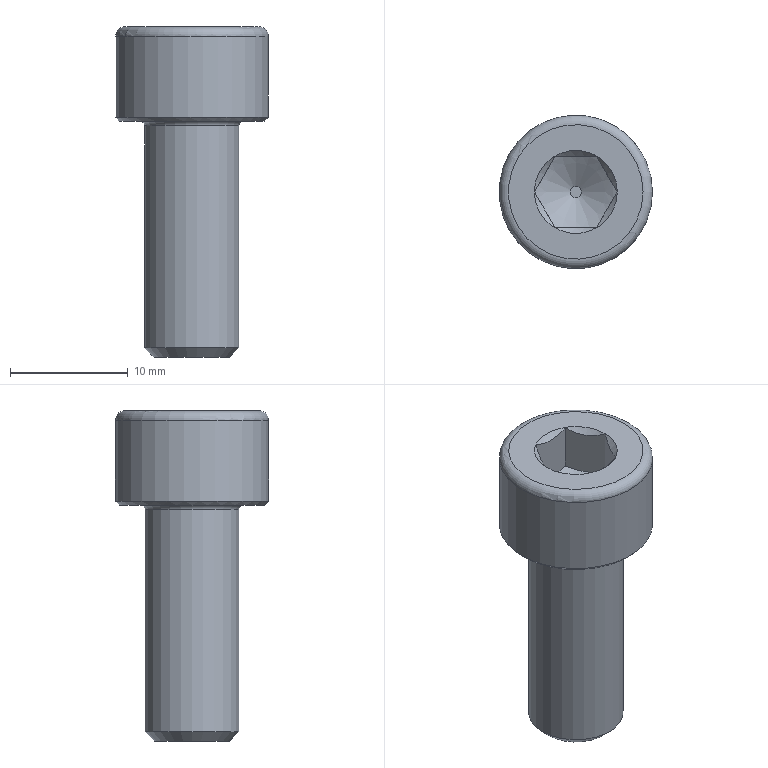Part | STEP file | Left | 1 solid | 18 faces | box 13 x 13 x 28 mm | volume 1899 mm3 | plane 10 | cone 4 | torus 2 | cylinder 2 | commonest cylinder face diameters 8 x1 13 x1
STEP:
#1=CARTESIAN_POINT('',(0.,0.,0.));
#2=DIRECTION('',(0.,0.,1.));
#3=DIRECTION('',(1.,0.,0.));
#4=AXIS2_PLACEMENT_3D('',#1,#2,#3);
#5=CARTESIAN_POINT('',(5.7,0.,8.));
#6=VERTEX_POINT('',#5);
#7=CARTESIAN_POINT('',(0.,0.,8.));
#8=DIRECTION('',(0.,0.,1.));
#9=DIRECTION('',(1.,0.,0.));
#10=AXIS2_PLACEMENT_3D('',#7,#8,#9);
#11=CIRCLE('',#10,5.7);
#12=CARTESIAN_POINT('',(0.,0.,8.));
#13=DIRECTION('',(0.,0.,1.));
#14=DIRECTION('',(1.,0.,0.));
#15=AXIS2_PLACEMENT_3D('',#12,#13,#14);
#16=PLANE('',#15);
#17=CARTESIAN_POINT('',(0.,0.));
#18=DIRECTION('',(1.,0.));
#19=AXIS2_PLACEMENT_2D('',#17,#18);
#20=CIRCLE('',#19,5.7);
#21=(GEOMETRIC_REPRESENTATION_CONTEXT(2)PARAMETRIC_REPRESENTATION_CONTEXT()REPRESENTATION_CONTEXT('',''));
#22=DEFINITIONAL_REPRESENTATION('',(#20),#21);
#23=PCURVE('',#16,#22);
#24=CARTESIAN_POINT('',(0.,0.,7.2));
#25=DIRECTION('',(0.,0.,-1.));
#26=DIRECTION('',(1.,0.,0.));
#27=AXIS2_PLACEMENT_3D('',#24,#25,#26);
#28=TOROIDAL_SURFACE('',#27,5.7,0.8);
#29=CARTESIAN_POINT('',(6.283,4.712));
#30=DIRECTION('',(-1.,0.));
#31=VECTOR('',#30,1.);
#32=LINE('',#29,#31);
#33=(GEOMETRIC_REPRESENTATION_CONTEXT(2)PARAMETRIC_REPRESENTATION_CONTEXT()REPRESENTATION_CONTEXT('',''));
#34=DEFINITIONAL_REPRESENTATION('',(#32),#33);
#35=PCURVE('',#28,#34);
#36=SURFACE_CURVE('',#11,(#23,#35),.PCURVE_S1.);
#37=EDGE_CURVE('',#6,#6,#36,.T.);
#38=ORIENTED_EDGE('',*,*,#37,.F.);
#39=EDGE_LOOP('',(#38));
#40=FACE_BOUND('',#39,.F.);
#41=CARTESIAN_POINT('',(-3.516,0.,8.));
#42=VERTEX_POINT('',#41);
#43=CARTESIAN_POINT('',(0.,0.,8.));
#44=DIRECTION('',(0.,0.,-1.));
#45=DIRECTION('',(-1.,0.,0.));
#46=AXIS2_PLACEMENT_3D('',#43,#44,#45);
#47=CIRCLE('',#46,3.516);
#48=CARTESIAN_POINT('',(-3.516,0.));
#49=CARTESIAN_POINT('',(-3.516,6.09));
#50=CARTESIAN_POINT('',(1.758,3.045));
#51=CARTESIAN_POINT('',(7.032,0.));
#52=CARTESIAN_POINT('',(1.758,-3.045));
#53=CARTESIAN_POINT('',(-3.516,-6.09));
#54=CARTESIAN_POINT('',(-3.516,0.));
#55=(BOUNDED_CURVE()B_SPLINE_CURVE(2,(#48,#49,#50,#51,#52,#53,#54),.UNSPECIFIED.,.T.,.F.)B_SPLINE_CURVE_WITH_KNOTS((1,2,2,2,2,1),(-2.094,0.,2.094,4.189,6.283,8.378),.UNSPECIFIED.)CURVE()GEOMETRIC_REPRESENTATION_ITEM()RATIONAL_B_SPLINE_CURVE((1.,0.5,1.,0.5,1.,0.5,1.))REPRESENTATION_ITEM(''));
#56=(GEOMETRIC_REPRESENTATION_CONTEXT(2)PARAMETRIC_REPRESENTATION_CONTEXT()REPRESENTATION_CONTEXT('',''));
#57=DEFINITIONAL_REPRESENTATION('',(#55),#56);
#58=PCURVE('',#16,#57);
#59=CARTESIAN_POINT('',(0.,0.,12.));
#60=DIRECTION('',(0.,0.,1.));
#61=DIRECTION('',(-1.,0.,0.));
#62=AXIS2_PLACEMENT_3D('',#59,#60,#61);
#63=CONICAL_SURFACE('',#62,7.516,0.7854);
#64=CARTESIAN_POINT('',(6.283,-4.));
#65=DIRECTION('',(-1.,0.));
#66=VECTOR('',#65,1.);
#67=LINE('',#64,#66);
#68=(GEOMETRIC_REPRESENTATION_CONTEXT(2)PARAMETRIC_REPRESENTATION_CONTEXT()REPRESENTATION_CONTEXT('',''));
#69=DEFINITIONAL_REPRESENTATION('',(#67),#68);
#70=PCURVE('',#63,#69);
#71=SURFACE_CURVE('',#47,(#58,#70),.PCURVE_S1.);
#72=EDGE_CURVE('',#42,#42,#71,.T.);
#73=ORIENTED_EDGE('',*,*,#72,.F.);
#74=EDGE_LOOP('',(#73));
#75=FACE_BOUND('',#74,.F.);
#76=ADVANCED_FACE('',(#40,#75),#16,.T.);
#77=CARTESIAN_POINT('',(6.5,0.,7.2));
#78=VERTEX_POINT('',#77);
#79=CARTESIAN_POINT('',(5.7,0.,7.2));
#80=DIRECTION('',(0.,1.,0.));
#81=DIRECTION('',(0.,0.,1.));
#82=AXIS2_PLACEMENT_3D('',#79,#80,#81);
#83=CIRCLE('',#82,0.8);
#84=CARTESIAN_POINT('',(6.283,4.712));
#85=DIRECTION('',(0.,1.));
#86=VECTOR('',#85,1.);
#87=LINE('',#84,#86);
#88=(GEOMETRIC_REPRESENTATION_CONTEXT(2)PARAMETRIC_REPRESENTATION_CONTEXT()REPRESENTATION_CONTEXT('',''));
#89=DEFINITIONAL_REPRESENTATION('',(#87),#88);
#90=PCURVE('',#28,#89);
#91=CARTESIAN_POINT('',(0.,4.712));
#92=DIRECTION('',(0.,1.));
#93=VECTOR('',#92,1.);
#94=LINE('',#91,#93);
#95=(GEOMETRIC_REPRESENTATION_CONTEXT(2)PARAMETRIC_REPRESENTATION_CONTEXT()REPRESENTATION_CONTEXT('',''));
#96=DEFINITIONAL_REPRESENTATION('',(#94),#95);
#97=PCURVE('',#28,#96);
#98=SEAM_CURVE('',#83,(#90,#97),.PCURVE_S1.);
#99=EDGE_CURVE('',#6,#78,#98,.T.);
#100=ORIENTED_EDGE('',*,*,#99,.T.);
#101=CARTESIAN_POINT('',(0.,0.,7.2));
#102=DIRECTION('',(0.,0.,1.));
#103=DIRECTION('',(1.,0.,0.));
#104=AXIS2_PLACEMENT_3D('',#101,#102,#103);
#105=CIRCLE('',#104,6.5);
#106=CARTESIAN_POINT('',(6.283,6.283));
#107=DIRECTION('',(-1.,0.));
#108=VECTOR('',#107,1.);
#109=LINE('',#106,#108);
#110=(GEOMETRIC_REPRESENTATION_CONTEXT(2)PARAMETRIC_REPRESENTATION_CONTEXT()REPRESENTATION_CONTEXT('',''));
#111=DEFINITIONAL_REPRESENTATION('',(#109),#110);
#112=PCURVE('',#28,#111);
#113=CARTESIAN_POINT('',(0.,0.,7.2));
#114=DIRECTION('',(0.,0.,-1.));
#115=DIRECTION('',(1.,0.,0.));
#116=AXIS2_PLACEMENT_3D('',#113,#114,#115);
#117=CYLINDRICAL_SURFACE('',#116,6.5);
#118=CARTESIAN_POINT('',(6.283,0.));
#119=DIRECTION('',(-1.,0.));
#120=VECTOR('',#119,1.);
#121=LINE('',#118,#120);
#122=(GEOMETRIC_REPRESENTATION_CONTEXT(2)PARAMETRIC_REPRESENTATION_CONTEXT()REPRESENTATION_CONTEXT('',''));
#123=DEFINITIONAL_REPRESENTATION('',(#121),#122);
#124=PCURVE('',#117,#123);
#125=SURFACE_CURVE('',#105,(#112,#124),.PCURVE_S1.);
#126=EDGE_CURVE('',#78,#78,#125,.T.);
#127=ORIENTED_EDGE('',*,*,#126,.T.);
#128=ORIENTED_EDGE('',*,*,#99,.F.);
#129=ORIENTED_EDGE('',*,*,#37,.F.);
#130=EDGE_LOOP('',(#100,#127,#128,#129));
#131=FACE_BOUND('',#130,.T.);
#132=ADVANCED_FACE('',(#131),#28,.T.);
#133=CARTESIAN_POINT('',(1.749,3.03,7.983));
#134=VERTEX_POINT('',#133);
#135=CARTESIAN_POINT('',(-1.749,3.03,7.983));
#136=VERTEX_POINT('',#135);
#137=CARTESIAN_POINT('',(0.,3.03,4.484));
#138=DIRECTION('',(0.,-1.,0.));
#139=DIRECTION('',(0.,0.,1.));
#140=AXIS2_PLACEMENT_3D('',#137,#138,#139);
#141=HYPERBOLA('',#140,3.03,3.03);
#142=CARTESIAN_POINT('',(4.189,-4.017));
#143=CARTESIAN_POINT('',(4.203,-4.047));
#144=CARTESIAN_POINT('',(4.232,-4.102));
#145=CARTESIAN_POINT('',(4.277,-4.176));
#146=CARTESIAN_POINT('',(4.323,-4.243));
#147=CARTESIAN_POINT('',(4.37,-4.301));
#148=CARTESIAN_POINT('',(4.417,-4.351));
#149=CARTESIAN_POINT('',(4.465,-4.393));
#150=CARTESIAN_POINT('',(4.514,-4.427));
#151=CARTESIAN_POINT('',(4.563,-4.453));
#152=CARTESIAN_POINT('',(4.613,-4.472));
#153=CARTESIAN_POINT('',(4.662,-4.484));
#154=CARTESIAN_POINT('',(4.712,-4.487));
#155=CARTESIAN_POINT('',(4.762,-4.484));
#156=CARTESIAN_POINT('',(4.812,-4.472));
#157=CARTESIAN_POINT('',(4.862,-4.453));
#158=CARTESIAN_POINT('',(4.911,-4.427));
#159=CARTESIAN_POINT('',(4.96,-4.393));
#160=CARTESIAN_POINT('',(5.008,-4.351));
#161=CARTESIAN_POINT('',(5.055,-4.301));
#162=CARTESIAN_POINT('',(5.102,-4.243));
#163=CARTESIAN_POINT('',(5.148,-4.176));
#164=CARTESIAN_POINT('',(5.192,-4.102));
#165=CARTESIAN_POINT('',(5.222,-4.047));
#166=CARTESIAN_POINT('',(5.236,-4.017));
#167=B_SPLINE_CURVE_WITH_KNOTS('',3,(#142,#143,#144,#145,#146,#147,#148,#149,#150,#151,#152,#153,#154,#155,#156,#157,#158,#159,#160,#161,#162,#163,#164,#165,#166),.UNSPECIFIED.,.F.,.F.,(4,1,1,1,1,1,1,1,1,1,1,1,1,1,1,1,1,1,1,1,1,1,4),(-0.5493,-0.4994,-0.4494,-0.3995,-0.3496,-0.2996,-0.2497,-0.1997,-0.1498,-0.09987,-0.04994,0.,0.04994,0.09987,0.1498,0.1997,0.2497,0.2996,0.3496,0.3995,0.4494,0.4994,0.5493),.UNSPECIFIED.);
#168=(GEOMETRIC_REPRESENTATION_CONTEXT(2)PARAMETRIC_REPRESENTATION_CONTEXT()REPRESENTATION_CONTEXT('',''));
#169=DEFINITIONAL_REPRESENTATION('',(#167),#168);
#170=PCURVE('',#63,#169);
#171=CARTESIAN_POINT('',(-1.749,3.03,12.));
#172=DIRECTION('',(0.,-1.,0.));
#173=DIRECTION('',(1.,0.,0.));
#174=AXIS2_PLACEMENT_3D('',#171,#172,#173);
#175=PLANE('',#174);
#176=CARTESIAN_POINT('',(1.749,-7.516));
#177=DIRECTION('',(0.,1.));
#178=AXIS2_PLACEMENT_2D('',#176,#177);
#179=HYPERBOLA('',#178,3.03,3.03);
#180=(GEOMETRIC_REPRESENTATION_CONTEXT(2)PARAMETRIC_REPRESENTATION_CONTEXT()REPRESENTATION_CONTEXT('',''));
#181=DEFINITIONAL_REPRESENTATION('',(#179),#180);
#182=PCURVE('',#175,#181);
#183=SURFACE_CURVE('',#141,(#170,#182),.PCURVE_S1.);
#184=EDGE_CURVE('',#134,#136,#183,.T.);
#185=ORIENTED_EDGE('',*,*,#184,.T.);
#186=CARTESIAN_POINT('',(-3.499,0.,7.983));
#187=VERTEX_POINT('',#186);
#188=CARTESIAN_POINT('',(-2.624,1.515,4.484));
#189=DIRECTION('',(0.866,-0.5,0.));
#190=DIRECTION('',(0.,0.,1.));
#191=AXIS2_PLACEMENT_3D('',#188,#189,#190);
#192=HYPERBOLA('',#191,3.03,3.03);
#193=CARTESIAN_POINT('',(5.236,-4.017));
#194=CARTESIAN_POINT('',(5.25,-4.047));
#195=CARTESIAN_POINT('',(5.28,-4.102));
#196=CARTESIAN_POINT('',(5.324,-4.176));
#197=CARTESIAN_POINT('',(5.37,-4.243));
#198=CARTESIAN_POINT('',(5.417,-4.301));
#199=CARTESIAN_POINT('',(5.464,-4.351));
#200=CARTESIAN_POINT('',(5.512,-4.393));
#201=CARTESIAN_POINT('',(5.561,-4.427));
#202=CARTESIAN_POINT('',(5.61,-4.453));
#203=CARTESIAN_POINT('',(5.66,-4.472));
#204=CARTESIAN_POINT('',(5.71,-4.484));
#205=CARTESIAN_POINT('',(5.76,-4.487));
#206=CARTESIAN_POINT('',(5.81,-4.484));
#207=CARTESIAN_POINT('',(5.859,-4.472));
#208=CARTESIAN_POINT('',(5.909,-4.453));
#209=CARTESIAN_POINT('',(5.958,-4.427));
#210=CARTESIAN_POINT('',(6.007,-4.393));
#211=CARTESIAN_POINT('',(6.055,-4.351));
#212=CARTESIAN_POINT('',(6.102,-4.301));
#213=CARTESIAN_POINT('',(6.149,-4.243));
#214=CARTESIAN_POINT('',(6.195,-4.176));
#215=CARTESIAN_POINT('',(6.24,-4.102));
#216=CARTESIAN_POINT('',(6.269,-4.047));
#217=CARTESIAN_POINT('',(6.283,-4.017));
#218=B_SPLINE_CURVE_WITH_KNOTS('',3,(#193,#194,#195,#196,#197,#198,#199,#200,#201,#202,#203,#204,#205,#206,#207,#208,#209,#210,#211,#212,#213,#214,#215,#216,#217),.UNSPECIFIED.,.F.,.F.,(4,1,1,1,1,1,1,1,1,1,1,1,1,1,1,1,1,1,1,1,1,1,4),(-0.5493,-0.4994,-0.4494,-0.3995,-0.3496,-0.2996,-0.2497,-0.1997,-0.1498,-0.09987,-0.04994,0.,0.04994,0.09987,0.1498,0.1997,0.2497,0.2996,0.3496,0.3995,0.4494,0.4994,0.5493),.UNSPECIFIED.);
#219=(GEOMETRIC_REPRESENTATION_CONTEXT(2)PARAMETRIC_REPRESENTATION_CONTEXT()REPRESENTATION_CONTEXT('',''));
#220=DEFINITIONAL_REPRESENTATION('',(#218),#219);
#221=PCURVE('',#63,#220);
#222=CARTESIAN_POINT('',(-3.499,0.,12.));
#223=DIRECTION('',(0.866,-0.5,0.));
#224=DIRECTION('',(0.5,0.866,0.));
#225=AXIS2_PLACEMENT_3D('',#222,#223,#224);
#226=PLANE('',#225);
#227=CARTESIAN_POINT('',(1.749,-7.516));
#228=DIRECTION('',(0.,1.));
#229=AXIS2_PLACEMENT_2D('',#227,#228);
#230=HYPERBOLA('',#229,3.03,3.03);
#231=(GEOMETRIC_REPRESENTATION_CONTEXT(2)PARAMETRIC_REPRESENTATION_CONTEXT()REPRESENTATION_CONTEXT('',''));
#232=DEFINITIONAL_REPRESENTATION('',(#230),#231);
#233=PCURVE('',#226,#232);
#234=SURFACE_CURVE('',#192,(#221,#233),.PCURVE_S1.);
#235=EDGE_CURVE('',#136,#187,#234,.T.);
#236=ORIENTED_EDGE('',*,*,#235,.T.);
#237=CARTESIAN_POINT('',(-7.516,0.,12.));
#238=DIRECTION('',(0.7071,0.,-0.7071));
#239=VECTOR('',#238,1.);
#240=LINE('',#237,#239);
#241=CARTESIAN_POINT('',(6.283,0.));
#242=DIRECTION('',(0.,-1.));
#243=VECTOR('',#242,1.);
#244=LINE('',#241,#243);
#245=(GEOMETRIC_REPRESENTATION_CONTEXT(2)PARAMETRIC_REPRESENTATION_CONTEXT()REPRESENTATION_CONTEXT('',''));
#246=DEFINITIONAL_REPRESENTATION('',(#244),#245);
#247=PCURVE('',#63,#246);
#248=CARTESIAN_POINT('',(0.,0.));
#249=DIRECTION('',(0.,-1.));
#250=VECTOR('',#249,1.);
#251=LINE('',#248,#250);
#252=(GEOMETRIC_REPRESENTATION_CONTEXT(2)PARAMETRIC_REPRESENTATION_CONTEXT()REPRESENTATION_CONTEXT('',''));
#253=DEFINITIONAL_REPRESENTATION('',(#251),#252);
#254=PCURVE('',#63,#253);
#255=SEAM_CURVE('',#240,(#247,#254),.PCURVE_S1.);
#256=EDGE_CURVE('',#42,#187,#255,.T.);
#257=ORIENTED_EDGE('',*,*,#256,.F.);
#258=ORIENTED_EDGE('',*,*,#72,.T.);
#259=ORIENTED_EDGE('',*,*,#256,.T.);
#260=CARTESIAN_POINT('',(-1.749,-3.03,7.983));
#261=VERTEX_POINT('',#260);
#262=CARTESIAN_POINT('',(-2.624,-1.515,4.484));
#263=DIRECTION('',(0.866,0.5,0.));
#264=DIRECTION('',(0.,0.,1.));
#265=AXIS2_PLACEMENT_3D('',#262,#263,#264);
#266=HYPERBOLA('',#265,3.03,3.03);
#267=CARTESIAN_POINT('',(0.,-4.017));
#268=CARTESIAN_POINT('',(0.01441,-4.047));
#269=CARTESIAN_POINT('',(0.04361,-4.102));
#270=CARTESIAN_POINT('',(0.08842,-4.176));
#271=CARTESIAN_POINT('',(0.1342,-4.243));
#272=CARTESIAN_POINT('',(0.1808,-4.301));
#273=CARTESIAN_POINT('',(0.2282,-4.351));
#274=CARTESIAN_POINT('',(0.2764,-4.393));
#275=CARTESIAN_POINT('',(0.3251,-4.427));
#276=CARTESIAN_POINT('',(0.3743,-4.453));
#277=CARTESIAN_POINT('',(0.4238,-4.472));
#278=CARTESIAN_POINT('',(0.4737,-4.484));
#279=CARTESIAN_POINT('',(0.5236,-4.487));
#280=CARTESIAN_POINT('',(0.5735,-4.484));
#281=CARTESIAN_POINT('',(0.6233,-4.472));
#282=CARTESIAN_POINT('',(0.6729,-4.453));
#283=CARTESIAN_POINT('',(0.7221,-4.427));
#284=CARTESIAN_POINT('',(0.7708,-4.393));
#285=CARTESIAN_POINT('',(0.819,-4.351));
#286=CARTESIAN_POINT('',(0.8664,-4.301));
#287=CARTESIAN_POINT('',(0.913,-4.243));
#288=CARTESIAN_POINT('',(0.9588,-4.176));
#289=CARTESIAN_POINT('',(1.004,-4.102));
#290=CARTESIAN_POINT('',(1.033,-4.047));
#291=CARTESIAN_POINT('',(1.047,-4.017));
#292=B_SPLINE_CURVE_WITH_KNOTS('',3,(#267,#268,#269,#270,#271,#272,#273,#274,#275,#276,#277,#278,#279,#280,#281,#282,#283,#284,#285,#286,#287,#288,#289,#290,#291),.UNSPECIFIED.,.F.,.F.,(4,1,1,1,1,1,1,1,1,1,1,1,1,1,1,1,1,1,1,1,1,1,4),(-0.5493,-0.4994,-0.4494,-0.3995,-0.3496,-0.2996,-0.2497,-0.1997,-0.1498,-0.09987,-0.04994,0.,0.04994,0.09987,0.1498,0.1997,0.2497,0.2996,0.3496,0.3995,0.4494,0.4994,0.5493),.UNSPECIFIED.);
#293=(GEOMETRIC_REPRESENTATION_CONTEXT(2)PARAMETRIC_REPRESENTATION_CONTEXT()REPRESENTATION_CONTEXT('',''));
#294=DEFINITIONAL_REPRESENTATION('',(#292),#293);
#295=PCURVE('',#63,#294);
#296=CARTESIAN_POINT('',(-1.749,-3.03,12.));
#297=DIRECTION('',(0.866,0.5,0.));
#298=DIRECTION('',(-0.5,0.866,0.));
#299=AXIS2_PLACEMENT_3D('',#296,#297,#298);
#300=PLANE('',#299);
#301=CARTESIAN_POINT('',(1.749,-7.516));
#302=DIRECTION('',(0.,1.));
#303=AXIS2_PLACEMENT_2D('',#301,#302);
#304=HYPERBOLA('',#303,3.03,3.03);
#305=(GEOMETRIC_REPRESENTATION_CONTEXT(2)PARAMETRIC_REPRESENTATION_CONTEXT()REPRESENTATION_CONTEXT('',''));
#306=DEFINITIONAL_REPRESENTATION('',(#304),#305);
#307=PCURVE('',#300,#306);
#308=SURFACE_CURVE('',#266,(#295,#307),.PCURVE_S1.);
#309=EDGE_CURVE('',#187,#261,#308,.T.);
#310=ORIENTED_EDGE('',*,*,#309,.T.);
#311=CARTESIAN_POINT('',(1.749,-3.03,7.983));
#312=VERTEX_POINT('',#311);
#313=CARTESIAN_POINT('',(0.,-3.03,4.484));
#314=DIRECTION('',(0.,1.,0.));
#315=DIRECTION('',(0.,0.,1.));
#316=AXIS2_PLACEMENT_3D('',#313,#314,#315);
#317=HYPERBOLA('',#316,3.03,3.03);
#318=CARTESIAN_POINT('',(1.047,-4.017));
#319=CARTESIAN_POINT('',(1.062,-4.047));
#320=CARTESIAN_POINT('',(1.091,-4.102));
#321=CARTESIAN_POINT('',(1.136,-4.176));
#322=CARTESIAN_POINT('',(1.181,-4.243));
#323=CARTESIAN_POINT('',(1.228,-4.301));
#324=CARTESIAN_POINT('',(1.275,-4.351));
#325=CARTESIAN_POINT('',(1.324,-4.393));
#326=CARTESIAN_POINT('',(1.372,-4.427));
#327=CARTESIAN_POINT('',(1.421,-4.453));
#328=CARTESIAN_POINT('',(1.471,-4.472));
#329=CARTESIAN_POINT('',(1.521,-4.484));
#330=CARTESIAN_POINT('',(1.571,-4.487));
#331=CARTESIAN_POINT('',(1.621,-4.484));
#332=CARTESIAN_POINT('',(1.671,-4.472));
#333=CARTESIAN_POINT('',(1.72,-4.453));
#334=CARTESIAN_POINT('',(1.769,-4.427));
#335=CARTESIAN_POINT('',(1.818,-4.393));
#336=CARTESIAN_POINT('',(1.866,-4.351));
#337=CARTESIAN_POINT('',(1.914,-4.301));
#338=CARTESIAN_POINT('',(1.96,-4.243));
#339=CARTESIAN_POINT('',(2.006,-4.176));
#340=CARTESIAN_POINT('',(2.051,-4.102));
#341=CARTESIAN_POINT('',(2.08,-4.047));
#342=CARTESIAN_POINT('',(2.094,-4.017));
#343=B_SPLINE_CURVE_WITH_KNOTS('',3,(#318,#319,#320,#321,#322,#323,#324,#325,#326,#327,#328,#329,#330,#331,#332,#333,#334,#335,#336,#337,#338,#339,#340,#341,#342),.UNSPECIFIED.,.F.,.F.,(4,1,1,1,1,1,1,1,1,1,1,1,1,1,1,1,1,1,1,1,1,1,4),(-0.5493,-0.4994,-0.4494,-0.3995,-0.3496,-0.2996,-0.2497,-0.1997,-0.1498,-0.09987,-0.04994,0.,0.04994,0.09987,0.1498,0.1997,0.2497,0.2996,0.3496,0.3995,0.4494,0.4994,0.5493),.UNSPECIFIED.);
#344=(GEOMETRIC_REPRESENTATION_CONTEXT(2)PARAMETRIC_REPRESENTATION_CONTEXT()REPRESENTATION_CONTEXT('',''));
#345=DEFINITIONAL_REPRESENTATION('',(#343),#344);
#346=PCURVE('',#63,#345);
#347=CARTESIAN_POINT('',(1.749,-3.03,12.));
#348=DIRECTION('',(0.,1.,0.));
#349=DIRECTION('',(-1.,0.,0.));
#350=AXIS2_PLACEMENT_3D('',#347,#348,#349);
#351=PLANE('',#350);
#352=CARTESIAN_POINT('',(1.749,-7.516));
#353=DIRECTION('',(0.,1.));
#354=AXIS2_PLACEMENT_2D('',#352,#353);
#355=HYPERBOLA('',#354,3.03,3.03);
#356=(GEOMETRIC_REPRESENTATION_CONTEXT(2)PARAMETRIC_REPRESENTATION_CONTEXT()REPRESENTATION_CONTEXT('',''));
#357=DEFINITIONAL_REPRESENTATION('',(#355),#356);
#358=PCURVE('',#351,#357);
#359=SURFACE_CURVE('',#317,(#346,#358),.PCURVE_S1.);
#360=EDGE_CURVE('',#261,#312,#359,.T.);
#361=ORIENTED_EDGE('',*,*,#360,.T.);
#362=CARTESIAN_POINT('',(3.499,0.,7.983));
#363=VERTEX_POINT('',#362);
#364=CARTESIAN_POINT('',(2.624,-1.515,4.484));
#365=DIRECTION('',(-0.866,0.5,0.));
#366=DIRECTION('',(0.,0.,1.));
#367=AXIS2_PLACEMENT_3D('',#364,#365,#366);
#368=HYPERBOLA('',#367,3.03,3.03);
#369=CARTESIAN_POINT('',(2.094,-4.017));
#370=CARTESIAN_POINT('',(2.109,-4.047));
#371=CARTESIAN_POINT('',(2.138,-4.102));
#372=CARTESIAN_POINT('',(2.183,-4.176));
#373=CARTESIAN_POINT('',(2.229,-4.243));
#374=CARTESIAN_POINT('',(2.275,-4.301));
#375=CARTESIAN_POINT('',(2.323,-4.351));
#376=CARTESIAN_POINT('',(2.371,-4.393));
#377=CARTESIAN_POINT('',(2.419,-4.427));
#378=CARTESIAN_POINT('',(2.469,-4.453));
#379=CARTESIAN_POINT('',(2.518,-4.472));
#380=CARTESIAN_POINT('',(2.568,-4.484));
#381=CARTESIAN_POINT('',(2.618,-4.487));
#382=CARTESIAN_POINT('',(2.668,-4.484));
#383=CARTESIAN_POINT('',(2.718,-4.472));
#384=CARTESIAN_POINT('',(2.767,-4.453));
#385=CARTESIAN_POINT('',(2.817,-4.427));
#386=CARTESIAN_POINT('',(2.865,-4.393));
#387=CARTESIAN_POINT('',(2.913,-4.351));
#388=CARTESIAN_POINT('',(2.961,-4.301));
#389=CARTESIAN_POINT('',(3.007,-4.243));
#390=CARTESIAN_POINT('',(3.053,-4.176));
#391=CARTESIAN_POINT('',(3.098,-4.102));
#392=CARTESIAN_POINT('',(3.127,-4.047));
#393=CARTESIAN_POINT('',(3.142,-4.017));
#394=B_SPLINE_CURVE_WITH_KNOTS('',3,(#369,#370,#371,#372,#373,#374,#375,#376,#377,#378,#379,#380,#381,#382,#383,#384,#385,#386,#387,#388,#389,#390,#391,#392,#393),.UNSPECIFIED.,.F.,.F.,(4,1,1,1,1,1,1,1,1,1,1,1,1,1,1,1,1,1,1,1,1,1,4),(-0.5493,-0.4994,-0.4494,-0.3995,-0.3496,-0.2996,-0.2497,-0.1997,-0.1498,-0.09987,-0.04994,0.,0.04994,0.09987,0.1498,0.1997,0.2497,0.2996,0.3496,0.3995,0.4494,0.4994,0.5493),.UNSPECIFIED.);
#395=(GEOMETRIC_REPRESENTATION_CONTEXT(2)PARAMETRIC_REPRESENTATION_CONTEXT()REPRESENTATION_CONTEXT('',''));
#396=DEFINITIONAL_REPRESENTATION('',(#394),#395);
#397=PCURVE('',#63,#396);
#398=CARTESIAN_POINT('',(3.499,0.,12.));
#399=DIRECTION('',(-0.866,0.5,0.));
#400=DIRECTION('',(-0.5,-0.866,0.));
#401=AXIS2_PLACEMENT_3D('',#398,#399,#400);
#402=PLANE('',#401);
#403=CARTESIAN_POINT('',(1.749,-7.516));
#404=DIRECTION('',(0.,1.));
#405=AXIS2_PLACEMENT_2D('',#403,#404);
#406=HYPERBOLA('',#405,3.03,3.03);
#407=(GEOMETRIC_REPRESENTATION_CONTEXT(2)PARAMETRIC_REPRESENTATION_CONTEXT()REPRESENTATION_CONTEXT('',''));
#408=DEFINITIONAL_REPRESENTATION('',(#406),#407);
#409=PCURVE('',#402,#408);
#410=SURFACE_CURVE('',#368,(#397,#409),.PCURVE_S1.);
#411=EDGE_CURVE('',#312,#363,#410,.T.);
#412=ORIENTED_EDGE('',*,*,#411,.T.);
#413=CARTESIAN_POINT('',(2.624,1.515,4.484));
#414=DIRECTION('',(-0.866,-0.5,0.));
#415=DIRECTION('',(0.,0.,1.));
#416=AXIS2_PLACEMENT_3D('',#413,#414,#415);
#417=HYPERBOLA('',#416,3.03,3.03);
#418=CARTESIAN_POINT('',(3.142,-4.017));
#419=CARTESIAN_POINT('',(3.156,-4.047));
#420=CARTESIAN_POINT('',(3.185,-4.102));
#421=CARTESIAN_POINT('',(3.23,-4.176));
#422=CARTESIAN_POINT('',(3.276,-4.243));
#423=CARTESIAN_POINT('',(3.322,-4.301));
#424=CARTESIAN_POINT('',(3.37,-4.351));
#425=CARTESIAN_POINT('',(3.418,-4.393));
#426=CARTESIAN_POINT('',(3.467,-4.427));
#427=CARTESIAN_POINT('',(3.516,-4.453));
#428=CARTESIAN_POINT('',(3.565,-4.472));
#429=CARTESIAN_POINT('',(3.615,-4.484));
#430=CARTESIAN_POINT('',(3.665,-4.487));
#431=CARTESIAN_POINT('',(3.715,-4.484));
#432=CARTESIAN_POINT('',(3.765,-4.472));
#433=CARTESIAN_POINT('',(3.815,-4.453));
#434=CARTESIAN_POINT('',(3.864,-4.427));
#435=CARTESIAN_POINT('',(3.912,-4.393));
#436=CARTESIAN_POINT('',(3.961,-4.351));
#437=CARTESIAN_POINT('',(4.008,-4.301));
#438=CARTESIAN_POINT('',(4.055,-4.243));
#439=CARTESIAN_POINT('',(4.1,-4.176));
#440=CARTESIAN_POINT('',(4.145,-4.102));
#441=CARTESIAN_POINT('',(4.174,-4.047));
#442=CARTESIAN_POINT('',(4.189,-4.017));
#443=B_SPLINE_CURVE_WITH_KNOTS('',3,(#418,#419,#420,#421,#422,#423,#424,#425,#426,#427,#428,#429,#430,#431,#432,#433,#434,#435,#436,#437,#438,#439,#440,#441,#442),.UNSPECIFIED.,.F.,.F.,(4,1,1,1,1,1,1,1,1,1,1,1,1,1,1,1,1,1,1,1,1,1,4),(-0.5493,-0.4994,-0.4494,-0.3995,-0.3496,-0.2996,-0.2497,-0.1997,-0.1498,-0.09987,-0.04994,0.,0.04994,0.09987,0.1498,0.1997,0.2497,0.2996,0.3496,0.3995,0.4494,0.4994,0.5493),.UNSPECIFIED.);
#444=(GEOMETRIC_REPRESENTATION_CONTEXT(2)PARAMETRIC_REPRESENTATION_CONTEXT()REPRESENTATION_CONTEXT('',''));
#445=DEFINITIONAL_REPRESENTATION('',(#443),#444);
#446=PCURVE('',#63,#445);
#447=CARTESIAN_POINT('',(1.749,3.03,12.));
#448=DIRECTION('',(-0.866,-0.5,0.));
#449=DIRECTION('',(0.5,-0.866,0.));
#450=AXIS2_PLACEMENT_3D('',#447,#448,#449);
#451=PLANE('',#450);
#452=CARTESIAN_POINT('',(1.749,-7.516));
#453=DIRECTION('',(0.,1.));
#454=AXIS2_PLACEMENT_2D('',#452,#453);
#455=HYPERBOLA('',#454,3.03,3.03);
#456=(GEOMETRIC_REPRESENTATION_CONTEXT(2)PARAMETRIC_REPRESENTATION_CONTEXT()REPRESENTATION_CONTEXT('',''));
#457=DEFINITIONAL_REPRESENTATION('',(#455),#456);
#458=PCURVE('',#451,#457);
#459=SURFACE_CURVE('',#417,(#446,#458),.PCURVE_S1.);
#460=EDGE_CURVE('',#363,#134,#459,.T.);
#461=ORIENTED_EDGE('',*,*,#460,.T.);
#462=EDGE_LOOP('',(#185,#236,#257,#258,#259,#310,#361,#412,#461));
#463=FACE_BOUND('',#462,.F.);
#464=ADVANCED_FACE('',(#463),#63,.F.);
#465=CARTESIAN_POINT('',(6.5,0.,0.335));
#466=VERTEX_POINT('',#465);
#467=CARTESIAN_POINT('',(6.5,0.,7.2));
#468=DIRECTION('',(0.,0.,-1.));
#469=VECTOR('',#468,1.);
#470=LINE('',#467,#469);
#471=CARTESIAN_POINT('',(6.283,0.));
#472=DIRECTION('',(0.,1.));
#473=VECTOR('',#472,1.);
#474=LINE('',#471,#473);
#475=(GEOMETRIC_REPRESENTATION_CONTEXT(2)PARAMETRIC_REPRESENTATION_CONTEXT()REPRESENTATION_CONTEXT('',''));
#476=DEFINITIONAL_REPRESENTATION('',(#474),#475);
#477=PCURVE('',#117,#476);
#478=CARTESIAN_POINT('',(0.,0.));
#479=DIRECTION('',(0.,1.));
#480=VECTOR('',#479,1.);
#481=LINE('',#478,#480);
#482=(GEOMETRIC_REPRESENTATION_CONTEXT(2)PARAMETRIC_REPRESENTATION_CONTEXT()REPRESENTATION_CONTEXT('',''));
#483=DEFINITIONAL_REPRESENTATION('',(#481),#482);
#484=PCURVE('',#117,#483);
#485=SEAM_CURVE('',#470,(#477,#484),.PCURVE_S1.);
#486=EDGE_CURVE('',#78,#466,#485,.T.);
#487=ORIENTED_EDGE('',*,*,#486,.T.);
#488=CARTESIAN_POINT('',(0.,0.,0.335));
#489=DIRECTION('',(0.,0.,1.));
#490=DIRECTION('',(1.,0.,0.));
#491=AXIS2_PLACEMENT_3D('',#488,#489,#490);
#492=CIRCLE('',#491,6.5);
#493=CARTESIAN_POINT('',(6.283,6.865));
#494=DIRECTION('',(-1.,0.));
#495=VECTOR('',#494,1.);
#496=LINE('',#493,#495);
#497=(GEOMETRIC_REPRESENTATION_CONTEXT(2)PARAMETRIC_REPRESENTATION_CONTEXT()REPRESENTATION_CONTEXT('',''));
#498=DEFINITIONAL_REPRESENTATION('',(#496),#497);
#499=PCURVE('',#117,#498);
#500=CARTESIAN_POINT('',(0.,0.,0.335));
#501=DIRECTION('',(0.,0.,1.));
#502=DIRECTION('',(1.,0.,0.));
#503=AXIS2_PLACEMENT_3D('',#500,#501,#502);
#504=CONICAL_SURFACE('',#503,6.5,0.7854);
#505=CARTESIAN_POINT('',(0.,0.));
#506=DIRECTION('',(1.,0.));
#507=VECTOR('',#506,1.);
#508=LINE('',#505,#507);
#509=(GEOMETRIC_REPRESENTATION_CONTEXT(2)PARAMETRIC_REPRESENTATION_CONTEXT()REPRESENTATION_CONTEXT('',''));
#510=DEFINITIONAL_REPRESENTATION('',(#508),#509);
#511=PCURVE('',#504,#510);
#512=SURFACE_CURVE('',#492,(#499,#511),.PCURVE_S1.);
#513=EDGE_CURVE('',#466,#466,#512,.T.);
#514=ORIENTED_EDGE('',*,*,#513,.T.);
#515=ORIENTED_EDGE('',*,*,#486,.F.);
#516=ORIENTED_EDGE('',*,*,#126,.F.);
#517=EDGE_LOOP('',(#487,#514,#515,#516));
#518=FACE_BOUND('',#517,.T.);
#519=ADVANCED_FACE('',(#518),#117,.T.);
#520=ORIENTED_EDGE('',*,*,#184,.T.);
#521=CARTESIAN_POINT('',(-1.749,3.03,4.));
#522=VERTEX_POINT('',#521);
#523=CARTESIAN_POINT('',(-1.749,3.03,12.));
#524=DIRECTION('',(0.,0.,-1.));
#525=VECTOR('',#524,1.);
#526=LINE('',#523,#525);
#527=CARTESIAN_POINT('',(0.,0.));
#528=DIRECTION('',(0.,-1.));
#529=VECTOR('',#528,1.);
#530=LINE('',#527,#529);
#531=(GEOMETRIC_REPRESENTATION_CONTEXT(2)PARAMETRIC_REPRESENTATION_CONTEXT()REPRESENTATION_CONTEXT('',''));
#532=DEFINITIONAL_REPRESENTATION('',(#530),#531);
#533=PCURVE('',#175,#532);
#534=CARTESIAN_POINT('',(3.499,0.));
#535=DIRECTION('',(0.,-1.));
#536=VECTOR('',#535,1.);
#537=LINE('',#534,#536);
#538=(GEOMETRIC_REPRESENTATION_CONTEXT(2)PARAMETRIC_REPRESENTATION_CONTEXT()REPRESENTATION_CONTEXT('',''));
#539=DEFINITIONAL_REPRESENTATION('',(#537),#538);
#540=PCURVE('',#226,#539);
#541=SURFACE_CURVE('',#526,(#533,#540),.PCURVE_S1.);
#542=EDGE_CURVE('',#136,#522,#541,.T.);
#543=ORIENTED_EDGE('',*,*,#542,.T.);
#544=CARTESIAN_POINT('',(1.749,3.03,4.));
#545=VERTEX_POINT('',#544);
#546=CARTESIAN_POINT('',(0.,3.03,1.98));
#547=DIRECTION('',(0.,-1.,0.));
#548=DIRECTION('',(0.,0.,1.));
#549=AXIS2_PLACEMENT_3D('',#546,#547,#548);
#550=HYPERBOLA('',#549,1.749,3.03);
#551=CARTESIAN_POINT('',(1.749,-10.02));
#552=DIRECTION('',(0.,1.));
#553=AXIS2_PLACEMENT_2D('',#551,#552);
#554=HYPERBOLA('',#553,1.749,3.03);
#555=(GEOMETRIC_REPRESENTATION_CONTEXT(2)PARAMETRIC_REPRESENTATION_CONTEXT()REPRESENTATION_CONTEXT('',''));
#556=DEFINITIONAL_REPRESENTATION('',(#554),#555);
#557=PCURVE('',#175,#556);
#558=CARTESIAN_POINT('',(0.,0.,12.));
#559=DIRECTION('',(0.,0.,1.));
#560=DIRECTION('',(-1.,0.,0.));
#561=AXIS2_PLACEMENT_3D('',#558,#559,#560);
#562=CONICAL_SURFACE('',#561,17.355,1.047);
#563=CARTESIAN_POINT('',(4.189,-8.));
#564=CARTESIAN_POINT('',(4.203,-8.017));
#565=CARTESIAN_POINT('',(4.232,-8.049));
#566=CARTESIAN_POINT('',(4.277,-8.092));
#567=CARTESIAN_POINT('',(4.323,-8.13));
#568=CARTESIAN_POINT('',(4.37,-8.163));
#569=CARTESIAN_POINT('',(4.417,-8.192));
#570=CARTESIAN_POINT('',(4.465,-8.217));
#571=CARTESIAN_POINT('',(4.514,-8.236));
#572=CARTESIAN_POINT('',(4.563,-8.252));
#573=CARTESIAN_POINT('',(4.613,-8.263));
#574=CARTESIAN_POINT('',(4.662,-8.269));
#575=CARTESIAN_POINT('',(4.712,-8.271));
#576=CARTESIAN_POINT('',(4.762,-8.269));
#577=CARTESIAN_POINT('',(4.812,-8.263));
#578=CARTESIAN_POINT('',(4.862,-8.252));
#579=CARTESIAN_POINT('',(4.911,-8.236));
#580=CARTESIAN_POINT('',(4.96,-8.217));
#581=CARTESIAN_POINT('',(5.008,-8.192));
#582=CARTESIAN_POINT('',(5.055,-8.163));
#583=CARTESIAN_POINT('',(5.102,-8.13));
#584=CARTESIAN_POINT('',(5.148,-8.092));
#585=CARTESIAN_POINT('',(5.192,-8.049));
#586=CARTESIAN_POINT('',(5.222,-8.017));
#587=CARTESIAN_POINT('',(5.236,-8.));
#588=B_SPLINE_CURVE_WITH_KNOTS('',3,(#563,#564,#565,#566,#567,#568,#569,#570,#571,#572,#573,#574,#575,#576,#577,#578,#579,#580,#581,#582,#583,#584,#585,#586,#587),.UNSPECIFIED.,.F.,.F.,(4,1,1,1,1,1,1,1,1,1,1,1,1,1,1,1,1,1,1,1,1,1,4),(-0.5493,-0.4994,-0.4494,-0.3995,-0.3496,-0.2996,-0.2497,-0.1997,-0.1498,-0.09987,-0.04994,0.,0.04994,0.09987,0.1498,0.1997,0.2497,0.2996,0.3496,0.3995,0.4494,0.4994,0.5493),.UNSPECIFIED.);
#589=(GEOMETRIC_REPRESENTATION_CONTEXT(2)PARAMETRIC_REPRESENTATION_CONTEXT()REPRESENTATION_CONTEXT('',''));
#590=DEFINITIONAL_REPRESENTATION('',(#588),#589);
#591=PCURVE('',#562,#590);
#592=SURFACE_CURVE('',#550,(#557,#591),.PCURVE_S1.);
#593=EDGE_CURVE('',#545,#522,#592,.T.);
#594=ORIENTED_EDGE('',*,*,#593,.F.);
#595=CARTESIAN_POINT('',(1.749,3.03,12.));
#596=DIRECTION('',(0.,0.,-1.));
#597=VECTOR('',#596,1.);
#598=LINE('',#595,#597);
#599=CARTESIAN_POINT('',(3.499,0.));
#600=DIRECTION('',(0.,-1.));
#601=VECTOR('',#600,1.);
#602=LINE('',#599,#601);
#603=(GEOMETRIC_REPRESENTATION_CONTEXT(2)PARAMETRIC_REPRESENTATION_CONTEXT()REPRESENTATION_CONTEXT('',''));
#604=DEFINITIONAL_REPRESENTATION('',(#602),#603);
#605=PCURVE('',#175,#604);
#606=CARTESIAN_POINT('',(0.,0.));
#607=DIRECTION('',(0.,-1.));
#608=VECTOR('',#607,1.);
#609=LINE('',#606,#608);
#610=(GEOMETRIC_REPRESENTATION_CONTEXT(2)PARAMETRIC_REPRESENTATION_CONTEXT()REPRESENTATION_CONTEXT('',''));
#611=DEFINITIONAL_REPRESENTATION('',(#609),#610);
#612=PCURVE('',#451,#611);
#613=SURFACE_CURVE('',#598,(#605,#612),.PCURVE_S1.);
#614=EDGE_CURVE('',#134,#545,#613,.T.);
#615=ORIENTED_EDGE('',*,*,#614,.F.);
#616=EDGE_LOOP('',(#520,#543,#594,#615));
#617=FACE_BOUND('',#616,.T.);
#618=ADVANCED_FACE('',(#617),#175,.T.);
#619=ORIENTED_EDGE('',*,*,#460,.T.);
#620=ORIENTED_EDGE('',*,*,#614,.T.);
#621=CARTESIAN_POINT('',(3.499,0.,4.));
#622=VERTEX_POINT('',#621);
#623=CARTESIAN_POINT('',(2.624,1.515,1.98));
#624=DIRECTION('',(-0.866,-0.5,0.));
#625=DIRECTION('',(0.,0.,1.));
#626=AXIS2_PLACEMENT_3D('',#623,#624,#625);
#627=HYPERBOLA('',#626,1.749,3.03);
#628=CARTESIAN_POINT('',(1.749,-10.02));
#629=DIRECTION('',(0.,1.));
#630=AXIS2_PLACEMENT_2D('',#628,#629);
#631=HYPERBOLA('',#630,1.749,3.03);
#632=(GEOMETRIC_REPRESENTATION_CONTEXT(2)PARAMETRIC_REPRESENTATION_CONTEXT()REPRESENTATION_CONTEXT('',''));
#633=DEFINITIONAL_REPRESENTATION('',(#631),#632);
#634=PCURVE('',#451,#633);
#635=CARTESIAN_POINT('',(3.142,-8.));
#636=CARTESIAN_POINT('',(3.156,-8.017));
#637=CARTESIAN_POINT('',(3.185,-8.049));
#638=CARTESIAN_POINT('',(3.23,-8.092));
#639=CARTESIAN_POINT('',(3.276,-8.13));
#640=CARTESIAN_POINT('',(3.322,-8.163));
#641=CARTESIAN_POINT('',(3.37,-8.192));
#642=CARTESIAN_POINT('',(3.418,-8.217));
#643=CARTESIAN_POINT('',(3.467,-8.236));
#644=CARTESIAN_POINT('',(3.516,-8.252));
#645=CARTESIAN_POINT('',(3.565,-8.263));
#646=CARTESIAN_POINT('',(3.615,-8.269));
#647=CARTESIAN_POINT('',(3.665,-8.271));
#648=CARTESIAN_POINT('',(3.715,-8.269));
#649=CARTESIAN_POINT('',(3.765,-8.263));
#650=CARTESIAN_POINT('',(3.815,-8.252));
#651=CARTESIAN_POINT('',(3.864,-8.236));
#652=CARTESIAN_POINT('',(3.912,-8.217));
#653=CARTESIAN_POINT('',(3.961,-8.192));
#654=CARTESIAN_POINT('',(4.008,-8.163));
#655=CARTESIAN_POINT('',(4.055,-8.13));
#656=CARTESIAN_POINT('',(4.1,-8.092));
#657=CARTESIAN_POINT('',(4.145,-8.049));
#658=CARTESIAN_POINT('',(4.174,-8.017));
#659=CARTESIAN_POINT('',(4.189,-8.));
#660=B_SPLINE_CURVE_WITH_KNOTS('',3,(#635,#636,#637,#638,#639,#640,#641,#642,#643,#644,#645,#646,#647,#648,#649,#650,#651,#652,#653,#654,#655,#656,#657,#658,#659),.UNSPECIFIED.,.F.,.F.,(4,1,1,1,1,1,1,1,1,1,1,1,1,1,1,1,1,1,1,1,1,1,4),(-0.5493,-0.4994,-0.4494,-0.3995,-0.3496,-0.2996,-0.2497,-0.1997,-0.1498,-0.09987,-0.04994,0.,0.04994,0.09987,0.1498,0.1997,0.2497,0.2996,0.3496,0.3995,0.4494,0.4994,0.5493),.UNSPECIFIED.);
#661=(GEOMETRIC_REPRESENTATION_CONTEXT(2)PARAMETRIC_REPRESENTATION_CONTEXT()REPRESENTATION_CONTEXT('',''));
#662=DEFINITIONAL_REPRESENTATION('',(#660),#661);
#663=PCURVE('',#562,#662);
#664=SURFACE_CURVE('',#627,(#634,#663),.PCURVE_S1.);
#665=EDGE_CURVE('',#622,#545,#664,.T.);
#666=ORIENTED_EDGE('',*,*,#665,.F.);
#667=CARTESIAN_POINT('',(3.499,0.,12.));
#668=DIRECTION('',(0.,0.,-1.));
#669=VECTOR('',#668,1.);
#670=LINE('',#667,#669);
#671=CARTESIAN_POINT('',(3.499,0.));
#672=DIRECTION('',(0.,-1.));
#673=VECTOR('',#672,1.);
#674=LINE('',#671,#673);
#675=(GEOMETRIC_REPRESENTATION_CONTEXT(2)PARAMETRIC_REPRESENTATION_CONTEXT()REPRESENTATION_CONTEXT('',''));
#676=DEFINITIONAL_REPRESENTATION('',(#674),#675);
#677=PCURVE('',#451,#676);
#678=CARTESIAN_POINT('',(0.,0.));
#679=DIRECTION('',(0.,-1.));
#680=VECTOR('',#679,1.);
#681=LINE('',#678,#680);
#682=(GEOMETRIC_REPRESENTATION_CONTEXT(2)PARAMETRIC_REPRESENTATION_CONTEXT()REPRESENTATION_CONTEXT('',''));
#683=DEFINITIONAL_REPRESENTATION('',(#681),#682);
#684=PCURVE('',#402,#683);
#685=SURFACE_CURVE('',#670,(#677,#684),.PCURVE_S1.);
#686=EDGE_CURVE('',#363,#622,#685,.T.);
#687=ORIENTED_EDGE('',*,*,#686,.F.);
#688=EDGE_LOOP('',(#619,#620,#666,#687));
#689=FACE_BOUND('',#688,.T.);
#690=ADVANCED_FACE('',(#689),#451,.T.);
#691=ORIENTED_EDGE('',*,*,#411,.T.);
#692=ORIENTED_EDGE('',*,*,#686,.T.);
#693=CARTESIAN_POINT('',(1.749,-3.03,4.));
#694=VERTEX_POINT('',#693);
#695=CARTESIAN_POINT('',(2.624,-1.515,1.98));
#696=DIRECTION('',(-0.866,0.5,0.));
#697=DIRECTION('',(0.,0.,1.));
#698=AXIS2_PLACEMENT_3D('',#695,#696,#697);
#699=HYPERBOLA('',#698,1.749,3.03);
#700=CARTESIAN_POINT('',(1.749,-10.02));
#701=DIRECTION('',(0.,1.));
#702=AXIS2_PLACEMENT_2D('',#700,#701);
#703=HYPERBOLA('',#702,1.749,3.03);
#704=(GEOMETRIC_REPRESENTATION_CONTEXT(2)PARAMETRIC_REPRESENTATION_CONTEXT()REPRESENTATION_CONTEXT('',''));
#705=DEFINITIONAL_REPRESENTATION('',(#703),#704);
#706=PCURVE('',#402,#705);
#707=CARTESIAN_POINT('',(2.094,-8.));
#708=CARTESIAN_POINT('',(2.109,-8.017));
#709=CARTESIAN_POINT('',(2.138,-8.049));
#710=CARTESIAN_POINT('',(2.183,-8.092));
#711=CARTESIAN_POINT('',(2.229,-8.13));
#712=CARTESIAN_POINT('',(2.275,-8.163));
#713=CARTESIAN_POINT('',(2.323,-8.192));
#714=CARTESIAN_POINT('',(2.371,-8.217));
#715=CARTESIAN_POINT('',(2.419,-8.236));
#716=CARTESIAN_POINT('',(2.469,-8.252));
#717=CARTESIAN_POINT('',(2.518,-8.263));
#718=CARTESIAN_POINT('',(2.568,-8.269));
#719=CARTESIAN_POINT('',(2.618,-8.271));
#720=CARTESIAN_POINT('',(2.668,-8.269));
#721=CARTESIAN_POINT('',(2.718,-8.263));
#722=CARTESIAN_POINT('',(2.767,-8.252));
#723=CARTESIAN_POINT('',(2.817,-8.236));
#724=CARTESIAN_POINT('',(2.865,-8.217));
#725=CARTESIAN_POINT('',(2.913,-8.192));
#726=CARTESIAN_POINT('',(2.961,-8.163));
#727=CARTESIAN_POINT('',(3.007,-8.13));
#728=CARTESIAN_POINT('',(3.053,-8.092));
#729=CARTESIAN_POINT('',(3.098,-8.049));
#730=CARTESIAN_POINT('',(3.127,-8.017));
#731=CARTESIAN_POINT('',(3.142,-8.));
#732=B_SPLINE_CURVE_WITH_KNOTS('',3,(#707,#708,#709,#710,#711,#712,#713,#714,#715,#716,#717,#718,#719,#720,#721,#722,#723,#724,#725,#726,#727,#728,#729,#730,#731),.UNSPECIFIED.,.F.,.F.,(4,1,1,1,1,1,1,1,1,1,1,1,1,1,1,1,1,1,1,1,1,1,4),(-0.5493,-0.4994,-0.4494,-0.3995,-0.3496,-0.2996,-0.2497,-0.1997,-0.1498,-0.09987,-0.04994,0.,0.04994,0.09987,0.1498,0.1997,0.2497,0.2996,0.3496,0.3995,0.4494,0.4994,0.5493),.QUASI_UNIFORM_KNOTS.);
#733=(GEOMETRIC_REPRESENTATION_CONTEXT(2)PARAMETRIC_REPRESENTATION_CONTEXT()REPRESENTATION_CONTEXT('',''));
#734=DEFINITIONAL_REPRESENTATION('',(#732),#733);
#735=PCURVE('',#562,#734);
#736=SURFACE_CURVE('',#699,(#706,#735),.PCURVE_S1.);
#737=EDGE_CURVE('',#694,#622,#736,.T.);
#738=ORIENTED_EDGE('',*,*,#737,.F.);
#739=CARTESIAN_POINT('',(1.749,-3.03,12.));
#740=DIRECTION('',(0.,0.,-1.));
#741=VECTOR('',#740,1.);
#742=LINE('',#739,#741);
#743=CARTESIAN_POINT('',(3.499,0.));
#744=DIRECTION('',(0.,-1.));
#745=VECTOR('',#744,1.);
#746=LINE('',#743,#745);
#747=(GEOMETRIC_REPRESENTATION_CONTEXT(2)PARAMETRIC_REPRESENTATION_CONTEXT()REPRESENTATION_CONTEXT('',''));
#748=DEFINITIONAL_REPRESENTATION('',(#746),#747);
#749=PCURVE('',#402,#748);
#750=CARTESIAN_POINT('',(0.,0.));
#751=DIRECTION('',(0.,-1.));
#752=VECTOR('',#751,1.);
#753=LINE('',#750,#752);
#754=(GEOMETRIC_REPRESENTATION_CONTEXT(2)PARAMETRIC_REPRESENTATION_CONTEXT()REPRESENTATION_CONTEXT('',''));
#755=DEFINITIONAL_REPRESENTATION('',(#753),#754);
#756=PCURVE('',#351,#755);
#757=SURFACE_CURVE('',#742,(#749,#756),.PCURVE_S1.);
#758=EDGE_CURVE('',#312,#694,#757,.T.);
#759=ORIENTED_EDGE('',*,*,#758,.F.);
#760=EDGE_LOOP('',(#691,#692,#738,#759));
#761=FACE_BOUND('',#760,.T.);
#762=ADVANCED_FACE('',(#761),#402,.T.);
#763=ORIENTED_EDGE('',*,*,#360,.T.);
#764=ORIENTED_EDGE('',*,*,#758,.T.);
#765=CARTESIAN_POINT('',(-1.749,-3.03,4.));
#766=VERTEX_POINT('',#765);
#767=CARTESIAN_POINT('',(0.,-3.03,1.98));
#768=DIRECTION('',(0.,1.,0.));
#769=DIRECTION('',(0.,0.,1.));
#770=AXIS2_PLACEMENT_3D('',#767,#768,#769);
#771=HYPERBOLA('',#770,1.749,3.03);
#772=CARTESIAN_POINT('',(1.749,-10.02));
#773=DIRECTION('',(0.,1.));
#774=AXIS2_PLACEMENT_2D('',#772,#773);
#775=HYPERBOLA('',#774,1.749,3.03);
#776=(GEOMETRIC_REPRESENTATION_CONTEXT(2)PARAMETRIC_REPRESENTATION_CONTEXT()REPRESENTATION_CONTEXT('',''));
#777=DEFINITIONAL_REPRESENTATION('',(#775),#776);
#778=PCURVE('',#351,#777);
#779=CARTESIAN_POINT('',(1.047,-8.));
#780=CARTESIAN_POINT('',(1.062,-8.017));
#781=CARTESIAN_POINT('',(1.091,-8.049));
#782=CARTESIAN_POINT('',(1.136,-8.092));
#783=CARTESIAN_POINT('',(1.181,-8.13));
#784=CARTESIAN_POINT('',(1.228,-8.163));
#785=CARTESIAN_POINT('',(1.275,-8.192));
#786=CARTESIAN_POINT('',(1.324,-8.217));
#787=CARTESIAN_POINT('',(1.372,-8.236));
#788=CARTESIAN_POINT('',(1.421,-8.252));
#789=CARTESIAN_POINT('',(1.471,-8.263));
#790=CARTESIAN_POINT('',(1.521,-8.269));
#791=CARTESIAN_POINT('',(1.571,-8.271));
#792=CARTESIAN_POINT('',(1.621,-8.269));
#793=CARTESIAN_POINT('',(1.671,-8.263));
#794=CARTESIAN_POINT('',(1.72,-8.252));
#795=CARTESIAN_POINT('',(1.769,-8.236));
#796=CARTESIAN_POINT('',(1.818,-8.217));
#797=CARTESIAN_POINT('',(1.866,-8.192));
#798=CARTESIAN_POINT('',(1.914,-8.163));
#799=CARTESIAN_POINT('',(1.96,-8.13));
#800=CARTESIAN_POINT('',(2.006,-8.092));
#801=CARTESIAN_POINT('',(2.051,-8.049));
#802=CARTESIAN_POINT('',(2.08,-8.017));
#803=CARTESIAN_POINT('',(2.094,-8.));
#804=B_SPLINE_CURVE_WITH_KNOTS('',3,(#779,#780,#781,#782,#783,#784,#785,#786,#787,#788,#789,#790,#791,#792,#793,#794,#795,#796,#797,#798,#799,#800,#801,#802,#803),.UNSPECIFIED.,.F.,.F.,(4,1,1,1,1,1,1,1,1,1,1,1,1,1,1,1,1,1,1,1,1,1,4),(-0.5493,-0.4994,-0.4494,-0.3995,-0.3496,-0.2996,-0.2497,-0.1997,-0.1498,-0.09987,-0.04994,0.,0.04994,0.09987,0.1498,0.1997,0.2497,0.2996,0.3496,0.3995,0.4494,0.4994,0.5493),.UNSPECIFIED.);
#805=(GEOMETRIC_REPRESENTATION_CONTEXT(2)PARAMETRIC_REPRESENTATION_CONTEXT()REPRESENTATION_CONTEXT('',''));
#806=DEFINITIONAL_REPRESENTATION('',(#804),#805);
#807=PCURVE('',#562,#806);
#808=SURFACE_CURVE('',#771,(#778,#807),.PCURVE_S1.);
#809=EDGE_CURVE('',#766,#694,#808,.T.);
#810=ORIENTED_EDGE('',*,*,#809,.F.);
#811=CARTESIAN_POINT('',(-1.749,-3.03,12.));
#812=DIRECTION('',(0.,0.,-1.));
#813=VECTOR('',#812,1.);
#814=LINE('',#811,#813);
#815=CARTESIAN_POINT('',(3.499,0.));
#816=DIRECTION('',(0.,-1.));
#817=VECTOR('',#816,1.);
#818=LINE('',#815,#817);
#819=(GEOMETRIC_REPRESENTATION_CONTEXT(2)PARAMETRIC_REPRESENTATION_CONTEXT()REPRESENTATION_CONTEXT('',''));
#820=DEFINITIONAL_REPRESENTATION('',(#818),#819);
#821=PCURVE('',#351,#820);
#822=CARTESIAN_POINT('',(0.,0.));
#823=DIRECTION('',(0.,-1.));
#824=VECTOR('',#823,1.);
#825=LINE('',#822,#824);
#826=(GEOMETRIC_REPRESENTATION_CONTEXT(2)PARAMETRIC_REPRESENTATION_CONTEXT()REPRESENTATION_CONTEXT('',''));
#827=DEFINITIONAL_REPRESENTATION('',(#825),#826);
#828=PCURVE('',#300,#827);
#829=SURFACE_CURVE('',#814,(#821,#828),.PCURVE_S1.);
#830=EDGE_CURVE('',#261,#766,#829,.T.);
#831=ORIENTED_EDGE('',*,*,#830,.F.);
#832=EDGE_LOOP('',(#763,#764,#810,#831));
#833=FACE_BOUND('',#832,.T.);
#834=ADVANCED_FACE('',(#833),#351,.T.);
#835=ORIENTED_EDGE('',*,*,#309,.T.);
#836=ORIENTED_EDGE('',*,*,#830,.T.);
#837=CARTESIAN_POINT('',(-3.499,0.,4.));
#838=VERTEX_POINT('',#837);
#839=CARTESIAN_POINT('',(-2.624,-1.515,1.98));
#840=DIRECTION('',(0.866,0.5,0.));
#841=DIRECTION('',(0.,0.,1.));
#842=AXIS2_PLACEMENT_3D('',#839,#840,#841);
#843=HYPERBOLA('',#842,1.749,3.03);
#844=CARTESIAN_POINT('',(1.749,-10.02));
#845=DIRECTION('',(0.,1.));
#846=AXIS2_PLACEMENT_2D('',#844,#845);
#847=HYPERBOLA('',#846,1.749,3.03);
#848=(GEOMETRIC_REPRESENTATION_CONTEXT(2)PARAMETRIC_REPRESENTATION_CONTEXT()REPRESENTATION_CONTEXT('',''));
#849=DEFINITIONAL_REPRESENTATION('',(#847),#848);
#850=PCURVE('',#300,#849);
#851=CARTESIAN_POINT('',(0.,-8.));
#852=CARTESIAN_POINT('',(0.01441,-8.017));
#853=CARTESIAN_POINT('',(0.04361,-8.049));
#854=CARTESIAN_POINT('',(0.08842,-8.092));
#855=CARTESIAN_POINT('',(0.1342,-8.13));
#856=CARTESIAN_POINT('',(0.1808,-8.163));
#857=CARTESIAN_POINT('',(0.2282,-8.192));
#858=CARTESIAN_POINT('',(0.2764,-8.217));
#859=CARTESIAN_POINT('',(0.3251,-8.236));
#860=CARTESIAN_POINT('',(0.3743,-8.252));
#861=CARTESIAN_POINT('',(0.4238,-8.263));
#862=CARTESIAN_POINT('',(0.4737,-8.269));
#863=CARTESIAN_POINT('',(0.5236,-8.271));
#864=CARTESIAN_POINT('',(0.5735,-8.269));
#865=CARTESIAN_POINT('',(0.6233,-8.263));
#866=CARTESIAN_POINT('',(0.6729,-8.252));
#867=CARTESIAN_POINT('',(0.7221,-8.236));
#868=CARTESIAN_POINT('',(0.7708,-8.217));
#869=CARTESIAN_POINT('',(0.819,-8.192));
#870=CARTESIAN_POINT('',(0.8664,-8.163));
#871=CARTESIAN_POINT('',(0.913,-8.13));
#872=CARTESIAN_POINT('',(0.9588,-8.092));
#873=CARTESIAN_POINT('',(1.004,-8.049));
#874=CARTESIAN_POINT('',(1.033,-8.017));
#875=CARTESIAN_POINT('',(1.047,-8.));
#876=B_SPLINE_CURVE_WITH_KNOTS('',3,(#851,#852,#853,#854,#855,#856,#857,#858,#859,#860,#861,#862,#863,#864,#865,#866,#867,#868,#869,#870,#871,#872,#873,#874,#875),.UNSPECIFIED.,.F.,.F.,(4,1,1,1,1,1,1,1,1,1,1,1,1,1,1,1,1,1,1,1,1,1,4),(-0.5493,-0.4994,-0.4494,-0.3995,-0.3496,-0.2996,-0.2497,-0.1997,-0.1498,-0.09987,-0.04994,0.,0.04994,0.09987,0.1498,0.1997,0.2497,0.2996,0.3496,0.3995,0.4494,0.4994,0.5493),.UNSPECIFIED.);
#877=(GEOMETRIC_REPRESENTATION_CONTEXT(2)PARAMETRIC_REPRESENTATION_CONTEXT()REPRESENTATION_CONTEXT('',''));
#878=DEFINITIONAL_REPRESENTATION('',(#876),#877);
#879=PCURVE('',#562,#878);
#880=SURFACE_CURVE('',#843,(#850,#879),.PCURVE_S1.);
#881=EDGE_CURVE('',#838,#766,#880,.T.);
#882=ORIENTED_EDGE('',*,*,#881,.F.);
#883=CARTESIAN_POINT('',(-3.499,0.,12.));
#884=DIRECTION('',(0.,0.,-1.));
#885=VECTOR('',#884,1.);
#886=LINE('',#883,#885);
#887=CARTESIAN_POINT('',(3.499,0.));
#888=DIRECTION('',(0.,-1.));
#889=VECTOR('',#888,1.);
#890=LINE('',#887,#889);
#891=(GEOMETRIC_REPRESENTATION_CONTEXT(2)PARAMETRIC_REPRESENTATION_CONTEXT()REPRESENTATION_CONTEXT('',''));
#892=DEFINITIONAL_REPRESENTATION('',(#890),#891);
#893=PCURVE('',#300,#892);
#894=CARTESIAN_POINT('',(0.,0.));
#895=DIRECTION('',(0.,-1.));
#896=VECTOR('',#895,1.);
#897=LINE('',#894,#896);
#898=(GEOMETRIC_REPRESENTATION_CONTEXT(2)PARAMETRIC_REPRESENTATION_CONTEXT()REPRESENTATION_CONTEXT('',''));
#899=DEFINITIONAL_REPRESENTATION('',(#897),#898);
#900=PCURVE('',#226,#899);
#901=SURFACE_CURVE('',#886,(#893,#900),.PCURVE_S1.);
#902=EDGE_CURVE('',#187,#838,#901,.T.);
#903=ORIENTED_EDGE('',*,*,#902,.F.);
#904=EDGE_LOOP('',(#835,#836,#882,#903));
#905=FACE_BOUND('',#904,.T.);
#906=ADVANCED_FACE('',(#905),#300,.T.);
#907=ORIENTED_EDGE('',*,*,#235,.T.);
#908=ORIENTED_EDGE('',*,*,#902,.T.);
#909=CARTESIAN_POINT('',(-2.624,1.515,1.98));
#910=DIRECTION('',(0.866,-0.5,0.));
#911=DIRECTION('',(0.,0.,1.));
#912=AXIS2_PLACEMENT_3D('',#909,#910,#911);
#913=HYPERBOLA('',#912,1.749,3.03);
#914=CARTESIAN_POINT('',(1.749,-10.02));
#915=DIRECTION('',(0.,1.));
#916=AXIS2_PLACEMENT_2D('',#914,#915);
#917=HYPERBOLA('',#916,1.749,3.03);
#918=(GEOMETRIC_REPRESENTATION_CONTEXT(2)PARAMETRIC_REPRESENTATION_CONTEXT()REPRESENTATION_CONTEXT('',''));
#919=DEFINITIONAL_REPRESENTATION('',(#917),#918);
#920=PCURVE('',#226,#919);
#921=CARTESIAN_POINT('',(5.236,-8.));
#922=CARTESIAN_POINT('',(5.25,-8.017));
#923=CARTESIAN_POINT('',(5.28,-8.049));
#924=CARTESIAN_POINT('',(5.324,-8.092));
#925=CARTESIAN_POINT('',(5.37,-8.13));
#926=CARTESIAN_POINT('',(5.417,-8.163));
#927=CARTESIAN_POINT('',(5.464,-8.192));
#928=CARTESIAN_POINT('',(5.512,-8.217));
#929=CARTESIAN_POINT('',(5.561,-8.236));
#930=CARTESIAN_POINT('',(5.61,-8.252));
#931=CARTESIAN_POINT('',(5.66,-8.263));
#932=CARTESIAN_POINT('',(5.71,-8.269));
#933=CARTESIAN_POINT('',(5.76,-8.271));
#934=CARTESIAN_POINT('',(5.81,-8.269));
#935=CARTESIAN_POINT('',(5.859,-8.263));
#936=CARTESIAN_POINT('',(5.909,-8.252));
#937=CARTESIAN_POINT('',(5.958,-8.236));
#938=CARTESIAN_POINT('',(6.007,-8.217));
#939=CARTESIAN_POINT('',(6.055,-8.192));
#940=CARTESIAN_POINT('',(6.102,-8.163));
#941=CARTESIAN_POINT('',(6.149,-8.13));
#942=CARTESIAN_POINT('',(6.195,-8.092));
#943=CARTESIAN_POINT('',(6.24,-8.049));
#944=CARTESIAN_POINT('',(6.269,-8.017));
#945=CARTESIAN_POINT('',(6.283,-8.));
#946=B_SPLINE_CURVE_WITH_KNOTS('',3,(#921,#922,#923,#924,#925,#926,#927,#928,#929,#930,#931,#932,#933,#934,#935,#936,#937,#938,#939,#940,#941,#942,#943,#944,#945),.UNSPECIFIED.,.F.,.F.,(4,1,1,1,1,1,1,1,1,1,1,1,1,1,1,1,1,1,1,1,1,1,4),(-0.5493,-0.4994,-0.4494,-0.3995,-0.3496,-0.2996,-0.2497,-0.1997,-0.1498,-0.09987,-0.04994,0.,0.04994,0.09987,0.1498,0.1997,0.2497,0.2996,0.3496,0.3995,0.4494,0.4994,0.5493),.UNSPECIFIED.);
#947=(GEOMETRIC_REPRESENTATION_CONTEXT(2)PARAMETRIC_REPRESENTATION_CONTEXT()REPRESENTATION_CONTEXT('',''));
#948=DEFINITIONAL_REPRESENTATION('',(#946),#947);
#949=PCURVE('',#562,#948);
#950=SURFACE_CURVE('',#913,(#920,#949),.PCURVE_S1.);
#951=EDGE_CURVE('',#522,#838,#950,.T.);
#952=ORIENTED_EDGE('',*,*,#951,.F.);
#953=ORIENTED_EDGE('',*,*,#542,.F.);
#954=EDGE_LOOP('',(#907,#908,#952,#953));
#955=FACE_BOUND('',#954,.T.);
#956=ADVANCED_FACE('',(#955),#226,.T.);
#957=CARTESIAN_POINT('',(6.165,0.,0.));
#958=VERTEX_POINT('',#957);
#959=CARTESIAN_POINT('',(6.5,0.,0.335));
#960=DIRECTION('',(-0.7071,0.,-0.7071));
#961=VECTOR('',#960,1.);
#962=LINE('',#959,#961);
#963=CARTESIAN_POINT('',(0.,0.));
#964=DIRECTION('',(0.,-1.));
#965=VECTOR('',#964,1.);
#966=LINE('',#963,#965);
#967=(GEOMETRIC_REPRESENTATION_CONTEXT(2)PARAMETRIC_REPRESENTATION_CONTEXT()REPRESENTATION_CONTEXT('',''));
#968=DEFINITIONAL_REPRESENTATION('',(#966),#967);
#969=PCURVE('',#504,#968);
#970=CARTESIAN_POINT('',(6.283,0.));
#971=DIRECTION('',(0.,-1.));
#972=VECTOR('',#971,1.);
#973=LINE('',#970,#972);
#974=(GEOMETRIC_REPRESENTATION_CONTEXT(2)PARAMETRIC_REPRESENTATION_CONTEXT()REPRESENTATION_CONTEXT('',''));
#975=DEFINITIONAL_REPRESENTATION('',(#973),#974);
#976=PCURVE('',#504,#975);
#977=SEAM_CURVE('',#962,(#969,#976),.PCURVE_S1.);
#978=EDGE_CURVE('',#466,#958,#977,.T.);
#979=ORIENTED_EDGE('',*,*,#978,.T.);
#980=CARTESIAN_POINT('',(0.,0.,0.));
#981=DIRECTION('',(0.,0.,1.));
#982=DIRECTION('',(1.,0.,0.));
#983=AXIS2_PLACEMENT_3D('',#980,#981,#982);
#984=CIRCLE('',#983,6.165);
#985=CARTESIAN_POINT('',(0.,-0.335));
#986=DIRECTION('',(1.,0.));
#987=VECTOR('',#986,1.);
#988=LINE('',#985,#987);
#989=(GEOMETRIC_REPRESENTATION_CONTEXT(2)PARAMETRIC_REPRESENTATION_CONTEXT()REPRESENTATION_CONTEXT('',''));
#990=DEFINITIONAL_REPRESENTATION('',(#988),#989);
#991=PCURVE('',#504,#990);
#992=CARTESIAN_POINT('',(0.,0.,0.));
#993=DIRECTION('',(0.,0.,1.));
#994=DIRECTION('',(1.,0.,0.));
#995=AXIS2_PLACEMENT_3D('',#992,#993,#994);
#996=PLANE('',#995);
#997=CARTESIAN_POINT('',(0.,0.));
#998=DIRECTION('',(1.,0.));
#999=AXIS2_PLACEMENT_2D('',#997,#998);
#1000=CIRCLE('',#999,6.165);
#1001=(GEOMETRIC_REPRESENTATION_CONTEXT(2)PARAMETRIC_REPRESENTATION_CONTEXT()REPRESENTATION_CONTEXT('',''));
#1002=DEFINITIONAL_REPRESENTATION('',(#1000),#1001);
#1003=PCURVE('',#996,#1002);
#1004=SURFACE_CURVE('',#984,(#991,#1003),.PCURVE_S1.);
#1005=EDGE_CURVE('',#958,#958,#1004,.T.);
#1006=ORIENTED_EDGE('',*,*,#1005,.T.);
#1007=ORIENTED_EDGE('',*,*,#978,.F.);
#1008=ORIENTED_EDGE('',*,*,#513,.F.);
#1009=EDGE_LOOP('',(#979,#1006,#1007,#1008));
#1010=FACE_BOUND('',#1009,.T.);
#1011=ADVANCED_FACE('',(#1010),#504,.T.);
#1012=CARTESIAN_POINT('',(-0.4848,0.,2.26));
#1013=VERTEX_POINT('',#1012);
#1014=CARTESIAN_POINT('',(-17.355,0.,12.));
#1015=DIRECTION('',(0.866,0.,-0.5));
#1016=VECTOR('',#1015,1.);
#1017=LINE('',#1014,#1016);
#1018=CARTESIAN_POINT('',(0.,0.));
#1019=DIRECTION('',(0.,-1.));
#1020=VECTOR('',#1019,1.);
#1021=LINE('',#1018,#1020);
#1022=(GEOMETRIC_REPRESENTATION_CONTEXT(2)PARAMETRIC_REPRESENTATION_CONTEXT()REPRESENTATION_CONTEXT('',''));
#1023=DEFINITIONAL_REPRESENTATION('',(#1021),#1022);
#1024=PCURVE('',#562,#1023);
#1025=CARTESIAN_POINT('',(6.283,0.));
#1026=DIRECTION('',(0.,-1.));
#1027=VECTOR('',#1026,1.);
#1028=LINE('',#1025,#1027);
#1029=(GEOMETRIC_REPRESENTATION_CONTEXT(2)PARAMETRIC_REPRESENTATION_CONTEXT()REPRESENTATION_CONTEXT('',''));
#1030=DEFINITIONAL_REPRESENTATION('',(#1028),#1029);
#1031=PCURVE('',#562,#1030);
#1032=SEAM_CURVE('',#1017,(#1024,#1031),.PCURVE_S1.);
#1033=EDGE_CURVE('',#838,#1013,#1032,.T.);
#1034=ORIENTED_EDGE('',*,*,#1033,.T.);
#1035=CARTESIAN_POINT('',(0.,0.,2.26));
#1036=DIRECTION('',(0.,0.,-1.));
#1037=DIRECTION('',(-1.,0.,0.));
#1038=AXIS2_PLACEMENT_3D('',#1035,#1036,#1037);
#1039=CIRCLE('',#1038,0.4848);
#1040=CARTESIAN_POINT('',(6.283,-9.74));
#1041=DIRECTION('',(-1.,0.));
#1042=VECTOR('',#1041,1.);
#1043=LINE('',#1040,#1042);
#1044=(GEOMETRIC_REPRESENTATION_CONTEXT(2)PARAMETRIC_REPRESENTATION_CONTEXT()REPRESENTATION_CONTEXT('',''));
#1045=DEFINITIONAL_REPRESENTATION('',(#1043),#1044);
#1046=PCURVE('',#562,#1045);
#1047=CARTESIAN_POINT('',(0.,0.,2.26));
#1048=DIRECTION('',(0.,0.,-1.));
#1049=DIRECTION('',(-1.,0.,0.));
#1050=AXIS2_PLACEMENT_3D('',#1047,#1048,#1049);
#1051=PLANE('',#1050);
#1052=CARTESIAN_POINT('',(0.,0.));
#1053=DIRECTION('',(1.,0.));
#1054=AXIS2_PLACEMENT_2D('',#1052,#1053);
#1055=CIRCLE('',#1054,0.4848);
#1056=(GEOMETRIC_REPRESENTATION_CONTEXT(2)PARAMETRIC_REPRESENTATION_CONTEXT()REPRESENTATION_CONTEXT('',''));
#1057=DEFINITIONAL_REPRESENTATION('',(#1055),#1056);
#1058=PCURVE('',#1051,#1057);
#1059=SURFACE_CURVE('',#1039,(#1046,#1058),.PCURVE_S1.);
#1060=EDGE_CURVE('',#1013,#1013,#1059,.T.);
#1061=ORIENTED_EDGE('',*,*,#1060,.F.);
#1062=ORIENTED_EDGE('',*,*,#1033,.F.);
#1063=ORIENTED_EDGE('',*,*,#951,.F.);
#1064=ORIENTED_EDGE('',*,*,#593,.F.);
#1065=ORIENTED_EDGE('',*,*,#665,.F.);
#1066=ORIENTED_EDGE('',*,*,#737,.F.);
#1067=ORIENTED_EDGE('',*,*,#809,.F.);
#1068=ORIENTED_EDGE('',*,*,#881,.F.);
#1069=EDGE_LOOP('',(#1034,#1061,#1062,#1063,#1064,#1065,#1066,#1067,#1068));
#1070=FACE_BOUND('',#1069,.F.);
#1071=ADVANCED_FACE('',(#1070),#562,.F.);
#1072=ORIENTED_EDGE('',*,*,#1005,.T.);
#1073=EDGE_LOOP('',(#1072));
#1074=FACE_BOUND('',#1073,.F.);
#1075=CARTESIAN_POINT('',(4.4,0.,0.));
#1076=VERTEX_POINT('',#1075);
#1077=CARTESIAN_POINT('',(0.,0.,0.));
#1078=DIRECTION('',(0.,0.,1.));
#1079=DIRECTION('',(1.,0.,0.));
#1080=AXIS2_PLACEMENT_3D('',#1077,#1078,#1079);
#1081=CIRCLE('',#1080,4.4);
#1082=CARTESIAN_POINT('',(0.,0.));
#1083=DIRECTION('',(1.,0.));
#1084=AXIS2_PLACEMENT_2D('',#1082,#1083);
#1085=CIRCLE('',#1084,4.4);
#1086=(GEOMETRIC_REPRESENTATION_CONTEXT(2)PARAMETRIC_REPRESENTATION_CONTEXT()REPRESENTATION_CONTEXT('',''));
#1087=DEFINITIONAL_REPRESENTATION('',(#1085),#1086);
#1088=PCURVE('',#996,#1087);
#1089=CARTESIAN_POINT('',(0.,0.,-0.4));
#1090=DIRECTION('',(0.,0.,1.));
#1091=DIRECTION('',(1.,0.,0.));
#1092=AXIS2_PLACEMENT_3D('',#1089,#1090,#1091);
#1093=TOROIDAL_SURFACE('',#1092,4.4,0.4);
#1094=CARTESIAN_POINT('',(0.,1.571));
#1095=DIRECTION('',(1.,0.));
#1096=VECTOR('',#1095,1.);
#1097=LINE('',#1094,#1096);
#1098=(GEOMETRIC_REPRESENTATION_CONTEXT(2)PARAMETRIC_REPRESENTATION_CONTEXT()REPRESENTATION_CONTEXT('',''));
#1099=DEFINITIONAL_REPRESENTATION('',(#1097),#1098);
#1100=PCURVE('',#1093,#1099);
#1101=SURFACE_CURVE('',#1081,(#1088,#1100),.PCURVE_S1.);
#1102=EDGE_CURVE('',#1076,#1076,#1101,.T.);
#1103=ORIENTED_EDGE('',*,*,#1102,.F.);
#1104=EDGE_LOOP('',(#1103));
#1105=FACE_BOUND('',#1104,.F.);
#1106=ADVANCED_FACE('',(#1074,#1105),#996,.F.);
#1107=ORIENTED_EDGE('',*,*,#1060,.T.);
#1108=EDGE_LOOP('',(#1107));
#1109=FACE_BOUND('',#1108,.F.);
#1110=ADVANCED_FACE('',(#1109),#1051,.F.);
#1111=ORIENTED_EDGE('',*,*,#1102,.T.);
#1112=CARTESIAN_POINT('',(4.,0.,-0.4));
#1113=VERTEX_POINT('',#1112);
#1114=CARTESIAN_POINT('',(4.4,0.,-0.4));
#1115=DIRECTION('',(0.,-1.,0.));
#1116=DIRECTION('',(0.,0.,1.));
#1117=AXIS2_PLACEMENT_3D('',#1114,#1115,#1116);
#1118=CIRCLE('',#1117,0.4);
#1119=CARTESIAN_POINT('',(6.283,1.571));
#1120=DIRECTION('',(0.,1.));
#1121=VECTOR('',#1120,1.);
#1122=LINE('',#1119,#1121);
#1123=(GEOMETRIC_REPRESENTATION_CONTEXT(2)PARAMETRIC_REPRESENTATION_CONTEXT()REPRESENTATION_CONTEXT('',''));
#1124=DEFINITIONAL_REPRESENTATION('',(#1122),#1123);
#1125=PCURVE('',#1093,#1124);
#1126=CARTESIAN_POINT('',(0.,1.571));
#1127=DIRECTION('',(0.,1.));
#1128=VECTOR('',#1127,1.);
#1129=LINE('',#1126,#1128);
#1130=(GEOMETRIC_REPRESENTATION_CONTEXT(2)PARAMETRIC_REPRESENTATION_CONTEXT()REPRESENTATION_CONTEXT('',''));
#1131=DEFINITIONAL_REPRESENTATION('',(#1129),#1130);
#1132=PCURVE('',#1093,#1131);
#1133=SEAM_CURVE('',#1118,(#1125,#1132),.PCURVE_S1.);
#1134=EDGE_CURVE('',#1076,#1113,#1133,.T.);
#1135=ORIENTED_EDGE('',*,*,#1134,.T.);
#1136=CARTESIAN_POINT('',(0.,0.,-0.4));
#1137=DIRECTION('',(0.,0.,1.));
#1138=DIRECTION('',(1.,0.,0.));
#1139=AXIS2_PLACEMENT_3D('',#1136,#1137,#1138);
#1140=CIRCLE('',#1139,4.);
#1141=CARTESIAN_POINT('',(0.,3.142));
#1142=DIRECTION('',(1.,0.));
#1143=VECTOR('',#1142,1.);
#1144=LINE('',#1141,#1143);
#1145=(GEOMETRIC_REPRESENTATION_CONTEXT(2)PARAMETRIC_REPRESENTATION_CONTEXT()REPRESENTATION_CONTEXT('',''));
#1146=DEFINITIONAL_REPRESENTATION('',(#1144),#1145);
#1147=PCURVE('',#1093,#1146);
#1148=CARTESIAN_POINT('',(0.,0.,-0.4));
#1149=DIRECTION('',(0.,0.,-1.));
#1150=DIRECTION('',(1.,0.,0.));
#1151=AXIS2_PLACEMENT_3D('',#1148,#1149,#1150);
#1152=CYLINDRICAL_SURFACE('',#1151,4.);
#1153=CARTESIAN_POINT('',(6.283,0.));
#1154=DIRECTION('',(-1.,0.));
#1155=VECTOR('',#1154,1.);
#1156=LINE('',#1153,#1155);
#1157=(GEOMETRIC_REPRESENTATION_CONTEXT(2)PARAMETRIC_REPRESENTATION_CONTEXT()REPRESENTATION_CONTEXT('',''));
#1158=DEFINITIONAL_REPRESENTATION('',(#1156),#1157);
#1159=PCURVE('',#1152,#1158);
#1160=SURFACE_CURVE('',#1140,(#1147,#1159),.PCURVE_S1.);
#1161=EDGE_CURVE('',#1113,#1113,#1160,.T.);
#1162=ORIENTED_EDGE('',*,*,#1161,.F.);
#1163=ORIENTED_EDGE('',*,*,#1134,.F.);
#1164=EDGE_LOOP('',(#1111,#1135,#1162,#1163));
#1165=FACE_BOUND('',#1164,.F.);
#1166=ADVANCED_FACE('',(#1165),#1093,.F.);
#1167=CARTESIAN_POINT('',(4.,0.,-19.2));
#1168=VERTEX_POINT('',#1167);
#1169=CARTESIAN_POINT('',(4.,0.,-0.4));
#1170=DIRECTION('',(0.,0.,-1.));
#1171=VECTOR('',#1170,1.);
#1172=LINE('',#1169,#1171);
#1173=CARTESIAN_POINT('',(6.283,0.));
#1174=DIRECTION('',(0.,1.));
#1175=VECTOR('',#1174,1.);
#1176=LINE('',#1173,#1175);
#1177=(GEOMETRIC_REPRESENTATION_CONTEXT(2)PARAMETRIC_REPRESENTATION_CONTEXT()REPRESENTATION_CONTEXT('',''));
#1178=DEFINITIONAL_REPRESENTATION('',(#1176),#1177);
#1179=PCURVE('',#1152,#1178);
#1180=CARTESIAN_POINT('',(0.,0.));
#1181=DIRECTION('',(0.,1.));
#1182=VECTOR('',#1181,1.);
#1183=LINE('',#1180,#1182);
#1184=(GEOMETRIC_REPRESENTATION_CONTEXT(2)PARAMETRIC_REPRESENTATION_CONTEXT()REPRESENTATION_CONTEXT('',''));
#1185=DEFINITIONAL_REPRESENTATION('',(#1183),#1184);
#1186=PCURVE('',#1152,#1185);
#1187=SEAM_CURVE('',#1172,(#1179,#1186),.PCURVE_S1.);
#1188=EDGE_CURVE('',#1113,#1168,#1187,.T.);
#1189=ORIENTED_EDGE('',*,*,#1188,.T.);
#1190=CARTESIAN_POINT('',(0.,0.,-19.2));
#1191=DIRECTION('',(0.,0.,1.));
#1192=DIRECTION('',(1.,0.,0.));
#1193=AXIS2_PLACEMENT_3D('',#1190,#1191,#1192);
#1194=CIRCLE('',#1193,4.);
#1195=CARTESIAN_POINT('',(6.283,18.8));
#1196=DIRECTION('',(-1.,0.));
#1197=VECTOR('',#1196,1.);
#1198=LINE('',#1195,#1197);
#1199=(GEOMETRIC_REPRESENTATION_CONTEXT(2)PARAMETRIC_REPRESENTATION_CONTEXT()REPRESENTATION_CONTEXT('',''));
#1200=DEFINITIONAL_REPRESENTATION('',(#1198),#1199);
#1201=PCURVE('',#1152,#1200);
#1202=CARTESIAN_POINT('',(0.,0.,-19.2));
#1203=DIRECTION('',(0.,0.,1.));
#1204=DIRECTION('',(1.,0.,0.));
#1205=AXIS2_PLACEMENT_3D('',#1202,#1203,#1204);
#1206=CONICAL_SURFACE('',#1205,4.,0.7854);
#1207=CARTESIAN_POINT('',(0.,0.));
#1208=DIRECTION('',(1.,0.));
#1209=VECTOR('',#1208,1.);
#1210=LINE('',#1207,#1209);
#1211=(GEOMETRIC_REPRESENTATION_CONTEXT(2)PARAMETRIC_REPRESENTATION_CONTEXT()REPRESENTATION_CONTEXT('',''));
#1212=DEFINITIONAL_REPRESENTATION('',(#1210),#1211);
#1213=PCURVE('',#1206,#1212);
#1214=SURFACE_CURVE('',#1194,(#1201,#1213),.PCURVE_S1.);
#1215=EDGE_CURVE('',#1168,#1168,#1214,.T.);
#1216=ORIENTED_EDGE('',*,*,#1215,.T.);
#1217=ORIENTED_EDGE('',*,*,#1188,.F.);
#1218=ORIENTED_EDGE('',*,*,#1161,.F.);
#1219=EDGE_LOOP('',(#1189,#1216,#1217,#1218));
#1220=FACE_BOUND('',#1219,.T.);
#1221=ADVANCED_FACE('',(#1220),#1152,.T.);
#1222=CARTESIAN_POINT('',(3.2,0.,-20.));
#1223=VERTEX_POINT('',#1222);
#1224=CARTESIAN_POINT('',(4.,0.,-19.2));
#1225=DIRECTION('',(-0.7071,0.,-0.7071));
#1226=VECTOR('',#1225,1.);
#1227=LINE('',#1224,#1226);
#1228=CARTESIAN_POINT('',(0.,0.));
#1229=DIRECTION('',(0.,-1.));
#1230=VECTOR('',#1229,1.);
#1231=LINE('',#1228,#1230);
#1232=(GEOMETRIC_REPRESENTATION_CONTEXT(2)PARAMETRIC_REPRESENTATION_CONTEXT()REPRESENTATION_CONTEXT('',''));
#1233=DEFINITIONAL_REPRESENTATION('',(#1231),#1232);
#1234=PCURVE('',#1206,#1233);
#1235=CARTESIAN_POINT('',(6.283,0.));
#1236=DIRECTION('',(0.,-1.));
#1237=VECTOR('',#1236,1.);
#1238=LINE('',#1235,#1237);
#1239=(GEOMETRIC_REPRESENTATION_CONTEXT(2)PARAMETRIC_REPRESENTATION_CONTEXT()REPRESENTATION_CONTEXT('',''));
#1240=DEFINITIONAL_REPRESENTATION('',(#1238),#1239);
#1241=PCURVE('',#1206,#1240);
#1242=SEAM_CURVE('',#1227,(#1234,#1241),.PCURVE_S1.);
#1243=EDGE_CURVE('',#1168,#1223,#1242,.T.);
#1244=ORIENTED_EDGE('',*,*,#1243,.T.);
#1245=CARTESIAN_POINT('',(0.,0.,-20.));
#1246=DIRECTION('',(0.,0.,1.));
#1247=DIRECTION('',(1.,0.,0.));
#1248=AXIS2_PLACEMENT_3D('',#1245,#1246,#1247);
#1249=CIRCLE('',#1248,3.2);
#1250=CARTESIAN_POINT('',(0.,-0.8));
#1251=DIRECTION('',(1.,0.));
#1252=VECTOR('',#1251,1.);
#1253=LINE('',#1250,#1252);
#1254=(GEOMETRIC_REPRESENTATION_CONTEXT(2)PARAMETRIC_REPRESENTATION_CONTEXT()REPRESENTATION_CONTEXT('',''));
#1255=DEFINITIONAL_REPRESENTATION('',(#1253),#1254);
#1256=PCURVE('',#1206,#1255);
#1257=CARTESIAN_POINT('',(0.,0.,-20.));
#1258=DIRECTION('',(0.,0.,1.));
#1259=DIRECTION('',(1.,0.,0.));
#1260=AXIS2_PLACEMENT_3D('',#1257,#1258,#1259);
#1261=PLANE('',#1260);
#1262=CARTESIAN_POINT('',(0.,0.));
#1263=DIRECTION('',(1.,0.));
#1264=AXIS2_PLACEMENT_2D('',#1262,#1263);
#1265=CIRCLE('',#1264,3.2);
#1266=(GEOMETRIC_REPRESENTATION_CONTEXT(2)PARAMETRIC_REPRESENTATION_CONTEXT()REPRESENTATION_CONTEXT('',''));
#1267=DEFINITIONAL_REPRESENTATION('',(#1265),#1266);
#1268=PCURVE('',#1261,#1267);
#1269=SURFACE_CURVE('',#1249,(#1256,#1268),.PCURVE_S1.);
#1270=EDGE_CURVE('',#1223,#1223,#1269,.T.);
#1271=ORIENTED_EDGE('',*,*,#1270,.T.);
#1272=ORIENTED_EDGE('',*,*,#1243,.F.);
#1273=ORIENTED_EDGE('',*,*,#1215,.F.);
#1274=EDGE_LOOP('',(#1244,#1271,#1272,#1273));
#1275=FACE_BOUND('',#1274,.T.);
#1276=ADVANCED_FACE('',(#1275),#1206,.T.);
#1277=ORIENTED_EDGE('',*,*,#1270,.T.);
#1278=EDGE_LOOP('',(#1277));
#1279=FACE_BOUND('',#1278,.F.);
#1280=ADVANCED_FACE('',(#1279),#1261,.F.);
#1281=CLOSED_SHELL('',(#76,#132,#464,#519,#618,#690,#762,#834,#906,#956,#1011,#1071,#1106,#1110,#1166,#1221,#1276,#1280));
#1282=MANIFOLD_SOLID_BREP('',#1281);
#1283=(LENGTH_UNIT()NAMED_UNIT(*)SI_UNIT(.MILLI.,.METRE.));
#1284=UNCERTAINTY_MEASURE_WITH_UNIT(LENGTH_MEASURE(0.0000001),#1283,'','');
#1285=(NAMED_UNIT(*)PLANE_ANGLE_UNIT()SI_UNIT($,.RADIAN.));
#1286=(NAMED_UNIT(*)SI_UNIT($,.STERADIAN.)SOLID_ANGLE_UNIT());
#1287=(GEOMETRIC_REPRESENTATION_CONTEXT(3)GLOBAL_UNCERTAINTY_ASSIGNED_CONTEXT((#1284))GLOBAL_UNIT_ASSIGNED_CONTEXT((#1283,#1285,#1286))REPRESENTATION_CONTEXT('',''));
#1288=ADVANCED_BREP_SHAPE_REPRESENTATION('',(#4,#1282),#1287);